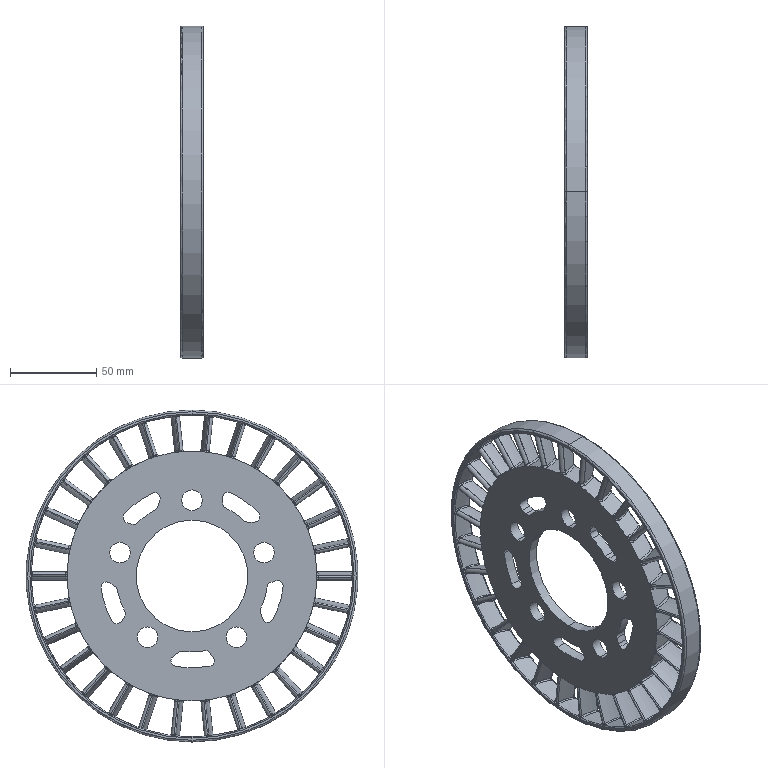Part | STEP file | Completa.sldasm-Part-26_Valor predeterminado | 1 solid | 949 faces | box 13.228 x 193 x 193 mm | volume 129234 mm3 | spline 540 | cylinder 321 | torus 73 | plane 15 | commonest cylinder face diameters 1 x60 4 x60 145 x31 187 x31 1.2 x30 53.531 x30